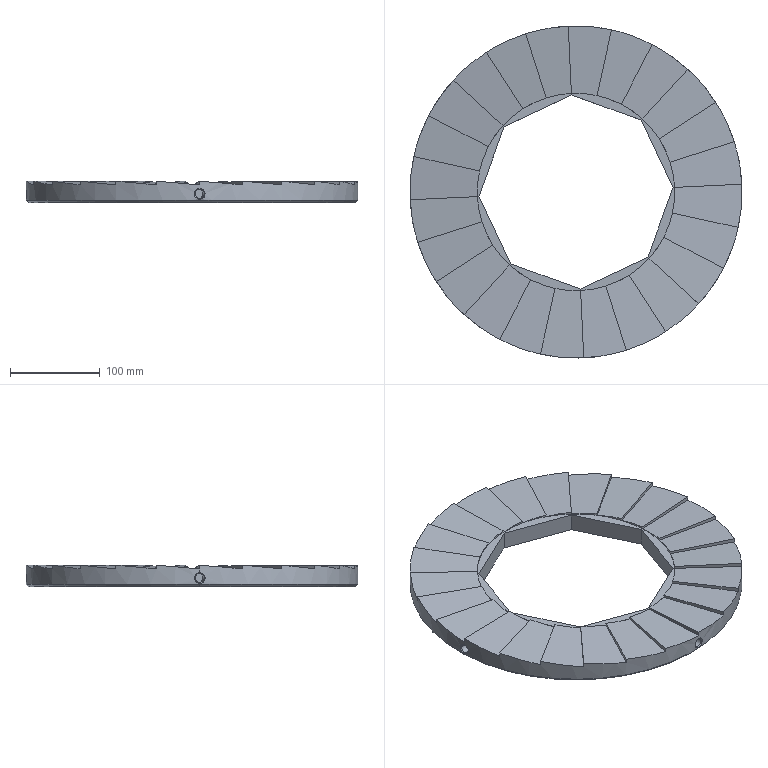Part | SolidWorks | features BaseBody 1 | 1 solid | 110 faces | box 370 x 370 x 24.255 mm | volume 1594243 mm3 | plane 62 | cylinder 35 | spline 11 | cone 2 | commonest cylinder face diameters 220 x25 10 x8 370 x2